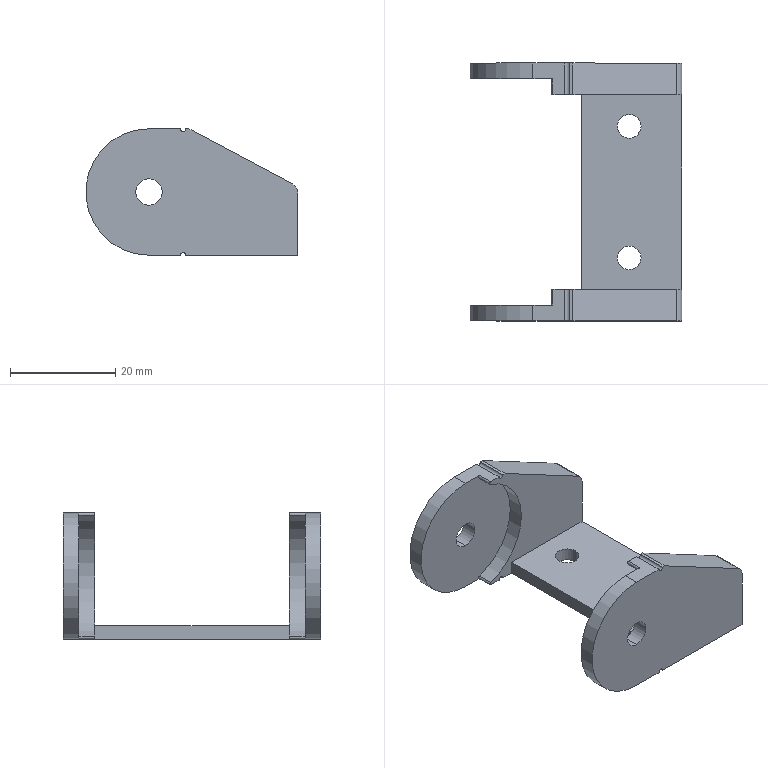Part | STEP file | 18_37_1 | 1 solid | 42 faces | box 40.3 x 49 x 24 mm | volume 8325 mm3 | cylinder 24 | plane 18 | commonest cylinder face diameters 1 x6 0.6 x4 4.5 x4 5 x4 24 x4 4 x2